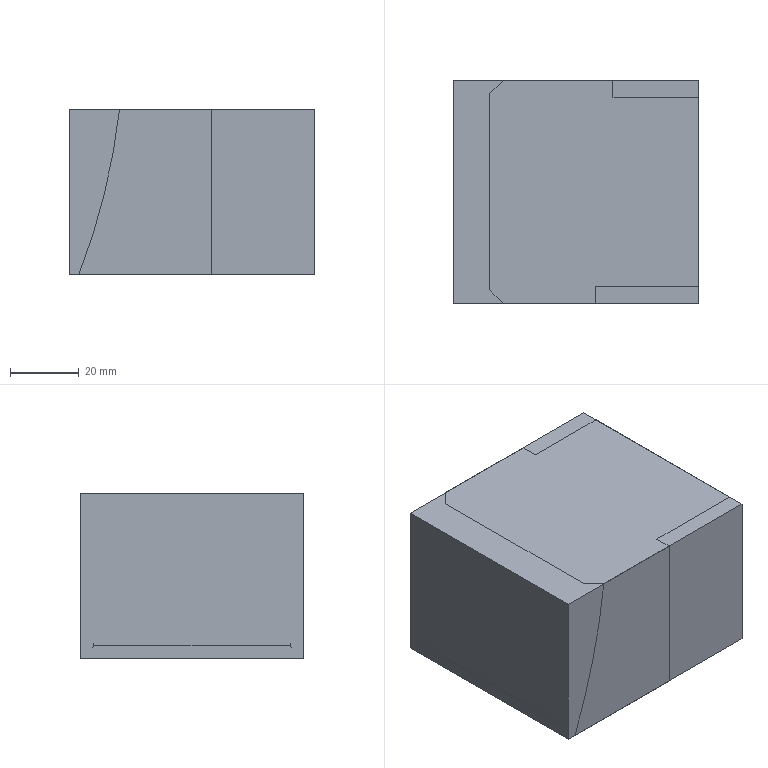NC program | NX | posted with a generic post | part box 71.51 x 65 x 48 mm
Whole program:
N10 G17 G21 G94 G90
(FLOOR_WALL_COPY , TOOL : D63)
N12 T01 M6
N14 G54
N16 G17 G0 G90 X-70.255 Y32.497 B0. C0. S6500 M3
N18 G43 Z30. H1
N20 Z7.
N22 G94 G1 Z4. F1250.
N24 X-67.255
N26 X67.255
N28 Y-7.3
N30 X-67.255
N32 X-70.255
N34 Z7.
N36 G0 Z30.
N38 Y32.497
N40 Z6.
N42 G1 Z3.
N44 X-67.255
N46 X67.255
N48 Y-7.3
N50 X-67.255
N52 X-70.255
N54 Z6.
N56 G0 Z30.
N58 Y32.497
N60 Z5.
N62 G1 Z2.
N64 X-67.255
N66 X67.255
N68 Y-7.3
N70 X-67.255
N72 X-70.255
N74 Z5.
N76 G0 Z30.
N78 Y32.497
N80 Z4.
N82 G1 Z1.
N84 X-67.255
N86 X67.255
N88 Y-7.3
N90 X-67.255
N92 X-70.255
N94 Z4.
N96 G0 Z30.
N98 Y32.497
N100 Z3.
N102 G1 Z0.
N104 X-67.255
N106 X67.255
N108 Y-7.3
N110 X-67.255
N112 X-70.255
N114 Z3.
N116 G0 Z30.
N118 M5
(ZLEVEL_PROFILE_1_COPY_1_COPY , TOOL : D6A45)
N120 T07 M6
N122 G54
N124 G17 G0 G90 X-36.676 Y34.453 B0. C0. S9500 M3
N126 G43 Z30. H7
N128 Z0.
N130 G94 G1 Z-1. F1000.
N132 X-36.275 Y33.759
N134 G3 X-35.756 Y33.459 R0.6
N136 G1 X35.756
N138 G2 X36.714 Y32.501 R0.958
N140 G1 Y-32.501
N142 G2 X35.756 Y-33.459 R0.958
N144 G1 X-35.756
N146 G2 X-36.714 Y-32.501 R0.958
N148 G1 Y32.501
N150 G2 X-35.756 Y33.459 R0.958
N152 G3 X-35.236 Y33.759 R0.6
N154 G1 X-34.717 Y34.659
N156 Z0.
N158 G0 Z30.
N160 M5
N162 M2